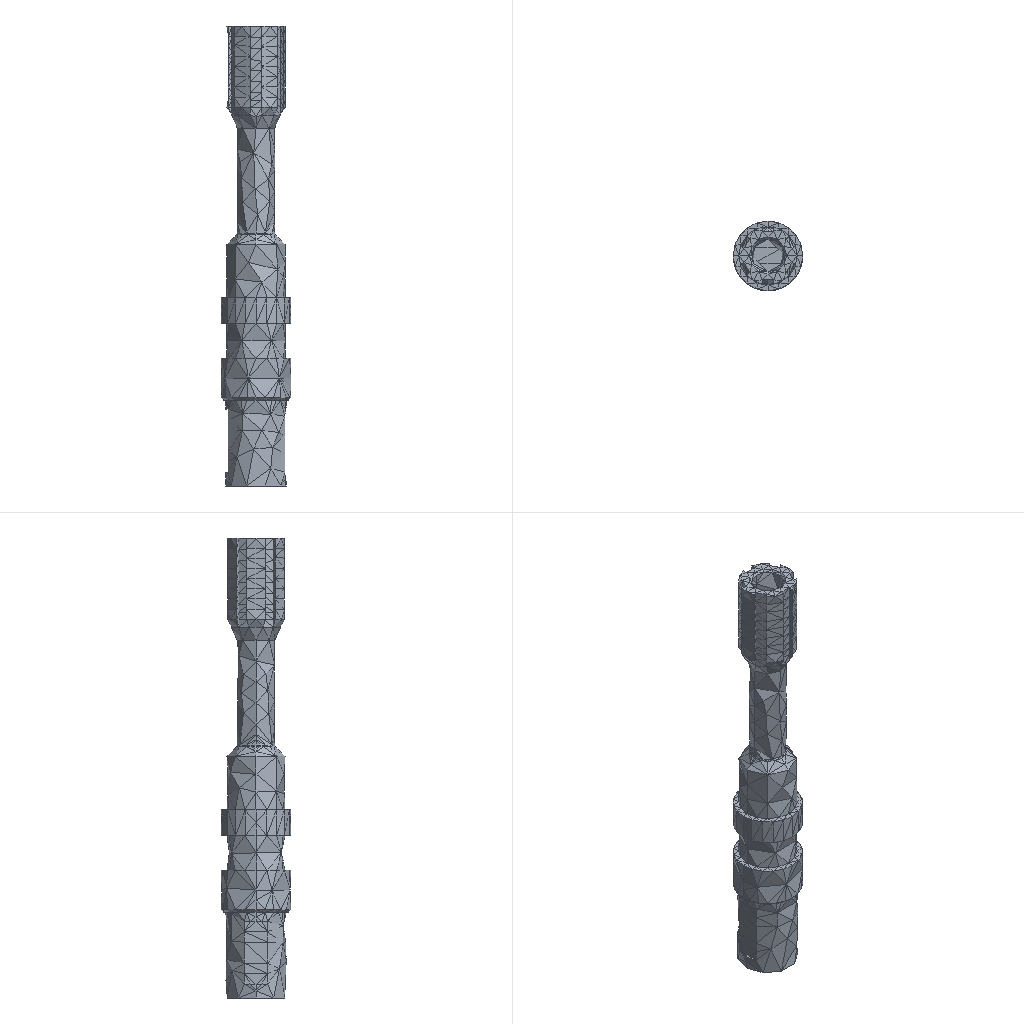Simulation study | ansys workbench
Ansys APDL input file, long lists of numbers shortened:
/batch
/config,noeldb,1     ! force off writing results to database
*get,_wallstrt,active,,time,wall
! ANSYS input file written by Workbench version 2022 R1
! File used for geometry attach: F:\ansys（分析文件汇总)\轴向柱塞泵有限元分析\轴向变量柱塞泵\轴向变量柱塞泵\驱动轴.STEP
/title,wbnew--__ (C5)
! ****** Begin Custom Load Command Snippet ******
/COM, ACT Extensions:
/COM,     LSDYNA, 2021.1
/COM,
! ****** End   Custom Load Command Snippet ******
*DIM,_wb_ProjectScratch_dir,string,248
_wb_ProjectScratch_dir(1) = 'C:\Users\Administrator\AppData\Local\Temp\WB_Administrator_15948_2\_ProjectScratch\Scr8355\'
*DIM,_wb_SolverFiles_dir,string,248
_wb_SolverFiles_dir(1) = 'C:\Users\Administrator\AppData\Local\Temp\WB_Administrator_15948_2\wbnew_files\dp0\SYS-1\MECH\'
*DIM,_wb_userfiles_dir,string,248
_wb_userfiles_dir(1) = 'C:\Users\Administrator\AppData\Local\Temp\WB_Administrator_15948_2\wbnew_files\user_files\'
/com,--- Data in consistent NMM units. See Solving Units in the help system for more information.
/units,MPA
/nopr
/wb,file,start              !  signify a WB generated input file
/prep7
! Turn off shape checking because checks already performed inside WB mesher.
! See help system for more information.
SHPP,OFF,,NOWARN
/nolist
etcon,set             ! allow ANSYS to choose best KEYOP's for 180x elements, resets any applicable keyopt to MAPDL defaults
/com,*********** Nodes for the whole assembly ***********
nblock,3,,5575
(1i9,3e20.9e3)
        1    -1.999999994E+00    -6.575305830E-08    -2.099100000E+02
! (5068 more lines like these left out)
-1
/wb,elem,start            !  set before creation of elements
/com,*********** Elements for Body 1 "___-FreeParts|prt0003.prt.2" ***********
et,1,187
eblock,19,solid,,2686
(19i9)
        1        1        1        1        0        0        0        0       10        0        1      123      847      437      364     1636     3637     1634     1633
! (5371 more lines like these left out)
-1
/wb,elem,end               !  done creating elements
/com,*********** Send User Defined Coordinate System(s) ***********
csys,0
toffst,273.15,  ! Temperature offset from absolute zero
/com,*********** Set Reference Temperature ***********
tref,22.
/wb,mat,start              !  starting to send materials
/com,*********** Send Materials ***********
Temperature = 'TEMP' ! Temperature
MP,DENS,1,7.85e-09,	! tonne mm^-3
MP,ALPX,1,1.2e-05,	! C^-1
MP,C,1,434000000,	! mm^2 s^-2 C^-1
MP,KXX,1,60.5,	! tonne mm s^-3 C^-1
MP,RSVX,1,0.00017,	! ohm mm
MP,EX,1,200000,	! tonne s^-2 mm^-1
MP,NUXY,1,0.3,
MP,MURX,1,10000,
/wb,mat,end                !  done sending materials
!************************* Model Summary ********************
!___-FreeParts|prt0003.prt.2,	结构钢,	matid,	1
!************************* End Model Summary ********************
! get the diagonal of the bounding box. Needed later for other things
*get,_xmin,node,,mnloc,x
*get,_ymin,node,,mnloc,y
*get,_zmin,node,,mnloc,z
*get,_xmax,node,,mxloc,x
*get,_ymax,node,,mxloc,y
*get,_zmax,node,,mxloc,z
_ASMDIAG=(_xmax-_xmin)*(_xmax-_xmin)+(_ymax-_ymin)*(_ymax-_ymin)+(_zmax-_zmin)*(_zmax-_zmin)
_ASMDIAG=SQRT(_ASMDIAG)
/wb,contact,start          !  starting to send contact
/wb,contact,end            !  done creating contacts
/golist
/wb,load,start             !  starting to send loads
/gst,on,on
fini
*get,_numnode,node,0,count
*get,_numelem,elem,0,count
*get, _MAXELEMNUM, elem, 0, NUM, MAX
*get, _MAXNODENUM, node, 0, NUM, MAX
*get, _MAXELEMTYPE, etyp, 0, NUM, MAX
*get, _MAXREALCONST, real, 0, NUM, MAX
/go
/wb,load,end               !  done creating loads
/com,--- Number of total nodes = %_numnode%
/com,--- Number of contact elements = 0
/com,--- Number of spring elements = 0
/com,--- Number of bearing elements = 0
/com,--- Number of solid elements = 2686
/com,--- Number of condensed parts = 0
/com,--- Number of total elements = %_numelem%
*get,_wallbsol,active,,time,wall
/solu
antype,2                   ! modal analysis
_thickRatio=  1     ! Ratio of thick parts in the model
modopt,lanb,12
outres,erase
outres,all,none
outres,nsol,all
outres,etmp,all
mxpand                    ! default expand in case of complex solution
dmpopt,esav,no
dmpopt,emat,no
dmpopt,full,no
! *********** WB SOLVE COMMAND ***********
! check interactive state
*get,ANSINTER_,active,,int
*if,ANSINTER_,ne,0,then
/eof
*endif
solve
/com *************** Write FE CONNECTORS *********
CEWRITE,file,ce,,INTE
*get,_nmodalsolproc,active,0,numcpu
fini
/nopr
*get,_numnode,node,0,count
*get,_numelem,elem,0,count
*get, _MAXELEMNUM, elem, 0, NUM, MAX
*get, _MAXNODENUM, node, 0, NUM, MAX,,,INTERNAL
*get, _MAXELEMTYPE, etyp, 0, NUM, MAX
*get, _MAXREALCONST, real, 0, NUM, MAX
/gopr
*get,_wallasol,active,,time,wall
/post1
/nopr
*dim,_direction,CHAR,6,1
_direction(1) = 'X'
_direction(2) = 'Y'
_direction(3) = 'Z'
_direction(4) = 'ROTX'
_direction(5) = 'ROTY'
_direction(6) = 'ROTZ'
*get,_lastLS,active,0,set,LSTP
*get,_beginset,active,0,set,nset,first,_lastLS
*get,_endset,active,0,set,nset,last,_lastLS
_nummodes = 0
*if,_endset,gt,0,then
_nummodes = _endset - _beginset + 1
*endif
*do,i_mode,1,_nummodes
   *do,j_component,1,6
			*get,PFACT_%i_mode%_%j_component%,MODE,%i_mode%,PFACT,,DIREC,_direction(%j_component%)
   *enddo
*enddo
*dim,_tmdirection,CHAR,6,1
_tmdirection(1) = 'X'
_tmdirection(2) = 'Y'
_tmdirection(3) = 'Z'
_tmdirection(4) = 'X'
_tmdirection(5) = 'Y'
_tmdirection(6) = 'Z'
*do,j_component,1,6
    *if,j_component,gt,3,then
        *get,TOTALMASS_%j_component%,ELEM,0,IOR,_tmdirection(%j_component%)
    *else
        *get,TOTALMASS_%j_component%,ELEM,0,MTOT,_tmdirection(%j_component%)
    *endif
*enddo
/gopr
xmlo,ENCODING,ISO-8859-1
xmlo,parm
/xml,parm,xml
fini
/gopr
*get,_walldone,active,,time,wall
_preptime=(_wallbsol-_wallstrt)*3600
_solvtime=(_wallasol-_wallbsol)*3600
_posttime=(_walldone-_wallasol)*3600
_totaltim=(_walldone-_wallstrt)*3600
*get,_dlbratio,active,0,solu,dlbr
*get,_combtime,active,0,solu,comb
*get,_ssmode,active,0,solu,ssmm
*get,_ndofs,active,0,solu,ndof
/fclean				!clean distributed files
/com,--- Total number of nodes = %_numnode%
/com,--- Total number of elements = %_numelem%
/com,--- Element load balance ratio = %_dlbratio%
/com,--- Time to combine distributed files = %_combtime%
/com,--- Sparse memory mode = %_ssmode%
/com,--- Number of DOF = %_ndofs%
/wb,file,end               ! done with WB generated input